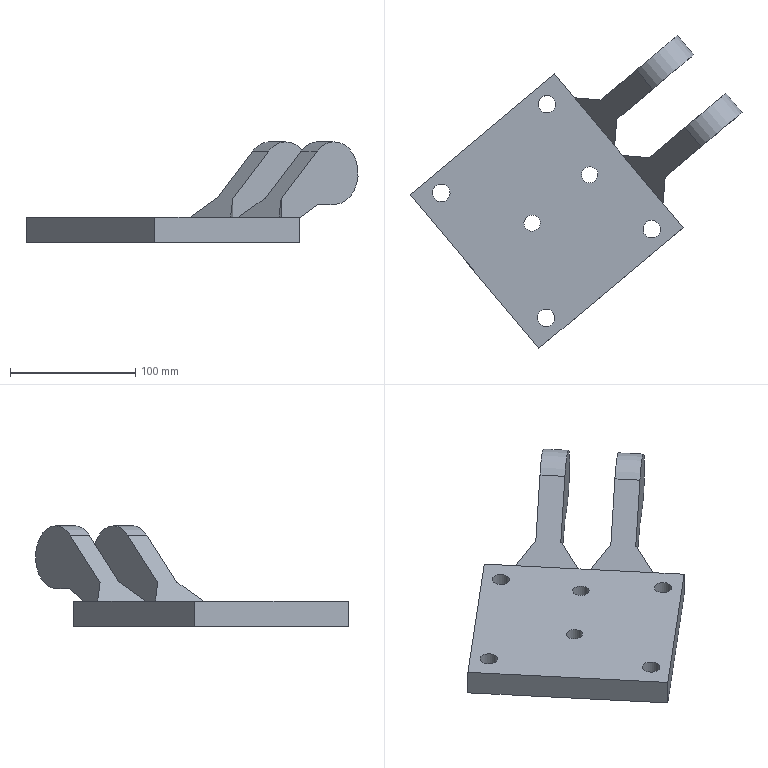Part | NX | features solid 2 | 1 solid | 30 faces | box 264.815 x 249.408 x 80 mm | volume 611339 mm3 | plane 22 | cylinder 8 | commonest cylinder face diameters 14 x4 13 x2 50 x2
STEP:
#1=CARTESIAN_POINT('',(922.471,361.992,-250.));
#2=VERTEX_POINT('',#1);
#3=CARTESIAN_POINT('',(906.401,381.143,-250.));
#4=VERTEX_POINT('',#3);
#5=CARTESIAN_POINT('',(977.108,296.878,-250.));
#6=DIRECTION('',(-0.6428,0.766,0.));
#7=VECTOR('',#6,1000.);
#8=LINE('',#5,#7);
#9=EDGE_CURVE('',#2,#4,#8,.T.);
#10=ORIENTED_EDGE('',*,*,#9,.T.);
#11=CARTESIAN_POINT('',(906.401,381.143,-230.));
#12=VERTEX_POINT('',#11);
#13=CARTESIAN_POINT('',(906.401,381.143,-230.));
#14=DIRECTION('',(0.,0.,1.));
#15=VECTOR('',#14,1000.);
#16=LINE('',#13,#15);
#17=EDGE_CURVE('',#4,#12,#16,.T.);
#18=ORIENTED_EDGE('',*,*,#17,.T.);
#19=CARTESIAN_POINT('',(922.471,361.992,-230.));
#20=VERTEX_POINT('',#19);
#21=CARTESIAN_POINT('',(977.108,296.878,-230.));
#22=DIRECTION('',(-0.6428,0.766,0.));
#23=VECTOR('',#22,1000.);
#24=LINE('',#21,#23);
#25=EDGE_CURVE('',#20,#12,#24,.T.);
#26=ORIENTED_EDGE('',*,*,#25,.F.);
#27=CARTESIAN_POINT('',(922.471,361.992,-230.));
#28=DIRECTION('',(0.,0.,-1.));
#29=VECTOR('',#28,1000.);
#30=LINE('',#27,#29);
#31=EDGE_CURVE('',#20,#2,#30,.T.);
#32=ORIENTED_EDGE('',*,*,#31,.T.);
#33=EDGE_LOOP('',(#10,#18,#26,#32));
#34=FACE_BOUND('',#33,.T.);
#35=CARTESIAN_POINT('',(977.108,296.878,-230.));
#36=DIRECTION('',(-0.766,-0.6428,0.));
#37=DIRECTION('',(0.,0.,-1.));
#38=AXIS2_PLACEMENT_3D('',#35,#36,#37);
#39=PLANE('',#38);
#40=ADVANCED_FACE('',(#34),#39,.F.);
#41=CARTESIAN_POINT('',(835.695,465.408,-230.));
#42=VERTEX_POINT('',#41);
#43=CARTESIAN_POINT('',(819.625,484.559,-230.));
#44=VERTEX_POINT('',#43);
#45=CARTESIAN_POINT('',(977.108,296.878,-230.));
#46=DIRECTION('',(-0.6428,0.766,0.));
#47=VECTOR('',#46,1000.);
#48=LINE('',#45,#47);
#49=EDGE_CURVE('',#42,#44,#48,.T.);
#50=ORIENTED_EDGE('',*,*,#49,.F.);
#51=CARTESIAN_POINT('',(835.695,465.408,-250.));
#52=VERTEX_POINT('',#51);
#53=CARTESIAN_POINT('',(835.695,465.408,-230.));
#54=DIRECTION('',(0.,0.,-1.));
#55=VECTOR('',#54,1000.);
#56=LINE('',#53,#55);
#57=EDGE_CURVE('',#42,#52,#56,.T.);
#58=ORIENTED_EDGE('',*,*,#57,.T.);
#59=CARTESIAN_POINT('',(819.625,484.559,-250.));
#60=VERTEX_POINT('',#59);
#61=CARTESIAN_POINT('',(977.108,296.878,-250.));
#62=DIRECTION('',(-0.6428,0.766,0.));
#63=VECTOR('',#62,1000.);
#64=LINE('',#61,#63);
#65=EDGE_CURVE('',#52,#60,#64,.T.);
#66=ORIENTED_EDGE('',*,*,#65,.T.);
#67=CARTESIAN_POINT('',(819.625,484.559,-230.));
#68=DIRECTION('',(0.,0.,-1.));
#69=VECTOR('',#68,1000.);
#70=LINE('',#67,#69);
#71=EDGE_CURVE('',#44,#60,#70,.T.);
#72=ORIENTED_EDGE('',*,*,#71,.F.);
#73=EDGE_LOOP('',(#50,#58,#66,#72));
#74=FACE_BOUND('',#73,.T.);
#75=CARTESIAN_POINT('',(977.108,296.878,-230.));
#76=DIRECTION('',(-0.766,-0.6428,0.));
#77=DIRECTION('',(0.,0.,-1.));
#78=AXIS2_PLACEMENT_3D('',#75,#76,#77);
#79=PLANE('',#78);
#80=ADVANCED_FACE('',(#74),#79,.F.);
#81=CARTESIAN_POINT('',(808.584,455.713,-230.));
#82=VERTEX_POINT('',#81);
#83=CARTESIAN_POINT('',(813.946,460.212,-230.));
#84=DIRECTION('',(0.,0.,1.));
#85=DIRECTION('',(-0.766,-0.6428,0.));
#86=AXIS2_PLACEMENT_3D('',#83,#84,#85);
#87=CIRCLE('',#86,7.);
#88=EDGE_CURVE('',#82,#82,#87,.T.);
#89=ORIENTED_EDGE('',*,*,#88,.F.);
#90=EDGE_LOOP('',(#89));
#91=FACE_BOUND('',#90,.T.);
#92=CARTESIAN_POINT('',(724.319,385.006,-230.));
#93=VERTEX_POINT('',#92);
#94=CARTESIAN_POINT('',(729.681,389.506,-230.));
#95=DIRECTION('',(0.,0.,1.));
#96=DIRECTION('',(-0.766,-0.6428,0.));
#97=AXIS2_PLACEMENT_3D('',#94,#95,#96);
#98=CIRCLE('',#97,7.);
#99=EDGE_CURVE('',#93,#93,#98,.T.);
#100=ORIENTED_EDGE('',*,*,#99,.F.);
#101=EDGE_LOOP('',(#100));
#102=FACE_BOUND('',#101,.T.);
#103=CARTESIAN_POINT('',(807.881,285.421,-230.));
#104=VERTEX_POINT('',#103);
#105=CARTESIAN_POINT('',(813.243,289.92,-230.));
#106=DIRECTION('',(0.,0.,1.));
#107=DIRECTION('',(-0.766,-0.6428,0.));
#108=AXIS2_PLACEMENT_3D('',#105,#106,#107);
#109=CIRCLE('',#108,7.);
#110=EDGE_CURVE('',#104,#104,#109,.T.);
#111=ORIENTED_EDGE('',*,*,#110,.F.);
#112=EDGE_LOOP('',(#111));
#113=FACE_BOUND('',#112,.T.);
#114=CARTESIAN_POINT('',(807.564,265.574,-230.));
#115=VERTEX_POINT('',#114);
#116=CARTESIAN_POINT('',(1251.87,638.39,-230.));
#117=DIRECTION('',(-0.766,-0.6428,0.));
#118=VECTOR('',#117,1000.);
#119=LINE('',#116,#118);
#120=EDGE_CURVE('',#20,#115,#119,.T.);
#121=ORIENTED_EDGE('',*,*,#120,.F.);
#122=ORIENTED_EDGE('',*,*,#25,.T.);
#123=CARTESIAN_POINT('',(874.262,419.445,-230.));
#124=VERTEX_POINT('',#123);
#125=CARTESIAN_POINT('',(896.759,392.634,-230.));
#126=DIRECTION('',(-0.6428,0.766,0.));
#127=VECTOR('',#126,1000.);
#128=LINE('',#125,#127);
#129=EDGE_CURVE('',#12,#124,#128,.T.);
#130=ORIENTED_EDGE('',*,*,#129,.T.);
#131=CARTESIAN_POINT('',(867.834,427.106,-230.));
#132=VERTEX_POINT('',#131);
#133=CARTESIAN_POINT('',(977.108,296.878,-230.));
#134=DIRECTION('',(-0.6428,0.766,0.));
#135=VECTOR('',#134,1000.);
#136=LINE('',#133,#135);
#137=EDGE_CURVE('',#124,#132,#136,.T.);
#138=ORIENTED_EDGE('',*,*,#137,.T.);
#139=CARTESIAN_POINT('',(858.192,438.596,-230.));
#140=DIRECTION('',(-0.6428,0.766,0.));
#141=VECTOR('',#140,1000.);
#142=LINE('',#139,#141);
#143=EDGE_CURVE('',#132,#42,#142,.T.);
#144=ORIENTED_EDGE('',*,*,#143,.T.);
#145=ORIENTED_EDGE('',*,*,#49,.T.);
#146=CARTESIAN_POINT('',(704.718,388.141,-230.));
#147=VERTEX_POINT('',#146);
#148=CARTESIAN_POINT('',(1149.024,760.958,-230.));
#149=DIRECTION('',(-0.766,-0.6428,0.));
#150=VECTOR('',#149,1000.);
#151=LINE('',#148,#150);
#152=EDGE_CURVE('',#44,#147,#151,.T.);
#153=ORIENTED_EDGE('',*,*,#152,.T.);
#154=CARTESIAN_POINT('',(862.201,200.46,-230.));
#155=DIRECTION('',(-0.6428,0.766,0.));
#156=VECTOR('',#155,1000.);
#157=LINE('',#154,#156);
#158=EDGE_CURVE('',#115,#147,#157,.T.);
#159=ORIENTED_EDGE('',*,*,#158,.F.);
#160=EDGE_LOOP('',(#121,#122,#130,#138,#144,#145,#153,#159));
#161=FACE_BOUND('',#160,.T.);
#162=CARTESIAN_POINT('',(797.125,361.246,-230.));
#163=VERTEX_POINT('',#162);
#164=CARTESIAN_POINT('',(802.104,365.424,-230.));
#165=DIRECTION('',(0.,0.,1.));
#166=DIRECTION('',(-0.766,-0.6428,0.));
#167=AXIS2_PLACEMENT_3D('',#164,#165,#166);
#168=CIRCLE('',#167,6.5);
#169=EDGE_CURVE('',#163,#163,#168,.T.);
#170=ORIENTED_EDGE('',*,*,#169,.F.);
#171=EDGE_LOOP('',(#170));
#172=FACE_BOUND('',#171,.T.);
#173=CARTESIAN_POINT('',(843.087,399.814,-230.));
#174=VERTEX_POINT('',#173);
#175=CARTESIAN_POINT('',(848.067,403.992,-230.));
#176=DIRECTION('',(0.,0.,1.));
#177=DIRECTION('',(-0.766,-0.6428,0.));
#178=AXIS2_PLACEMENT_3D('',#175,#176,#177);
#179=CIRCLE('',#178,6.5);
#180=EDGE_CURVE('',#174,#174,#179,.T.);
#181=ORIENTED_EDGE('',*,*,#180,.F.);
#182=EDGE_LOOP('',(#181));
#183=FACE_BOUND('',#182,.T.);
#184=CARTESIAN_POINT('',(892.146,356.127,-230.));
#185=VERTEX_POINT('',#184);
#186=CARTESIAN_POINT('',(897.508,360.627,-230.));
#187=DIRECTION('',(0.,0.,1.));
#188=DIRECTION('',(-0.766,-0.6428,0.));
#189=AXIS2_PLACEMENT_3D('',#186,#187,#188);
#190=CIRCLE('',#189,7.);
#191=EDGE_CURVE('',#185,#185,#190,.T.);
#192=ORIENTED_EDGE('',*,*,#191,.F.);
#193=EDGE_LOOP('',(#192));
#194=FACE_BOUND('',#193,.T.);
#195=CARTESIAN_POINT('',(1062.923,476.582,-230.));
#196=DIRECTION('',(0.,0.,1.));
#197=DIRECTION('',(-0.766,-0.6428,0.));
#198=AXIS2_PLACEMENT_3D('',#195,#196,#197);
#199=PLANE('',#198);
#200=ADVANCED_FACE('',(#91,#102,#113,#161,#172,#183,#194),#199,.T.);
#201=CARTESIAN_POINT('',(808.584,455.713,-250.));
#202=VERTEX_POINT('',#201);
#203=CARTESIAN_POINT('',(813.946,460.212,-250.));
#204=DIRECTION('',(0.,0.,1.));
#205=DIRECTION('',(-0.766,-0.6428,0.));
#206=AXIS2_PLACEMENT_3D('',#203,#204,#205);
#207=CIRCLE('',#206,7.);
#208=EDGE_CURVE('',#202,#202,#207,.T.);
#209=ORIENTED_EDGE('',*,*,#208,.T.);
#210=EDGE_LOOP('',(#209));
#211=FACE_BOUND('',#210,.T.);
#212=CARTESIAN_POINT('',(724.319,385.006,-250.));
#213=VERTEX_POINT('',#212);
#214=CARTESIAN_POINT('',(729.681,389.506,-250.));
#215=DIRECTION('',(0.,0.,1.));
#216=DIRECTION('',(-0.766,-0.6428,0.));
#217=AXIS2_PLACEMENT_3D('',#214,#215,#216);
#218=CIRCLE('',#217,7.);
#219=EDGE_CURVE('',#213,#213,#218,.T.);
#220=ORIENTED_EDGE('',*,*,#219,.T.);
#221=EDGE_LOOP('',(#220));
#222=FACE_BOUND('',#221,.T.);
#223=CARTESIAN_POINT('',(807.881,285.421,-250.));
#224=VERTEX_POINT('',#223);
#225=CARTESIAN_POINT('',(813.243,289.92,-250.));
#226=DIRECTION('',(0.,0.,1.));
#227=DIRECTION('',(-0.766,-0.6428,0.));
#228=AXIS2_PLACEMENT_3D('',#225,#226,#227);
#229=CIRCLE('',#228,7.);
#230=EDGE_CURVE('',#224,#224,#229,.T.);
#231=ORIENTED_EDGE('',*,*,#230,.T.);
#232=EDGE_LOOP('',(#231));
#233=FACE_BOUND('',#232,.T.);
#234=CARTESIAN_POINT('',(807.564,265.574,-250.));
#235=VERTEX_POINT('',#234);
#236=CARTESIAN_POINT('',(1251.87,638.39,-250.));
#237=DIRECTION('',(-0.766,-0.6428,0.));
#238=VECTOR('',#237,1000.);
#239=LINE('',#236,#238);
#240=EDGE_CURVE('',#2,#235,#239,.T.);
#241=ORIENTED_EDGE('',*,*,#240,.T.);
#242=CARTESIAN_POINT('',(704.718,388.141,-250.));
#243=VERTEX_POINT('',#242);
#244=CARTESIAN_POINT('',(862.201,200.46,-250.));
#245=DIRECTION('',(-0.6428,0.766,0.));
#246=VECTOR('',#245,1000.);
#247=LINE('',#244,#246);
#248=EDGE_CURVE('',#235,#243,#247,.T.);
#249=ORIENTED_EDGE('',*,*,#248,.T.);
#250=CARTESIAN_POINT('',(1149.024,760.958,-250.));
#251=DIRECTION('',(-0.766,-0.6428,0.));
#252=VECTOR('',#251,1000.);
#253=LINE('',#250,#252);
#254=EDGE_CURVE('',#60,#243,#253,.T.);
#255=ORIENTED_EDGE('',*,*,#254,.F.);
#256=ORIENTED_EDGE('',*,*,#65,.F.);
#257=CARTESIAN_POINT('',(867.834,427.106,-250.));
#258=VERTEX_POINT('',#257);
#259=CARTESIAN_POINT('',(858.192,438.596,-250.));
#260=DIRECTION('',(-0.6428,0.766,0.));
#261=VECTOR('',#260,1000.);
#262=LINE('',#259,#261);
#263=EDGE_CURVE('',#258,#52,#262,.T.);
#264=ORIENTED_EDGE('',*,*,#263,.F.);
#265=CARTESIAN_POINT('',(874.262,419.445,-250.));
#266=VERTEX_POINT('',#265);
#267=CARTESIAN_POINT('',(977.108,296.878,-250.));
#268=DIRECTION('',(-0.6428,0.766,0.));
#269=VECTOR('',#268,1000.);
#270=LINE('',#267,#269);
#271=EDGE_CURVE('',#266,#258,#270,.T.);
#272=ORIENTED_EDGE('',*,*,#271,.F.);
#273=CARTESIAN_POINT('',(896.759,392.634,-250.));
#274=DIRECTION('',(-0.6428,0.766,0.));
#275=VECTOR('',#274,1000.);
#276=LINE('',#273,#275);
#277=EDGE_CURVE('',#4,#266,#276,.T.);
#278=ORIENTED_EDGE('',*,*,#277,.F.);
#279=ORIENTED_EDGE('',*,*,#9,.F.);
#280=EDGE_LOOP('',(#241,#249,#255,#256,#264,#272,#278,#279));
#281=FACE_BOUND('',#280,.T.);
#282=CARTESIAN_POINT('',(797.125,361.246,-250.));
#283=VERTEX_POINT('',#282);
#284=CARTESIAN_POINT('',(802.104,365.424,-250.));
#285=DIRECTION('',(0.,0.,1.));
#286=DIRECTION('',(-0.766,-0.6428,0.));
#287=AXIS2_PLACEMENT_3D('',#284,#285,#286);
#288=CIRCLE('',#287,6.5);
#289=EDGE_CURVE('',#283,#283,#288,.T.);
#290=ORIENTED_EDGE('',*,*,#289,.T.);
#291=EDGE_LOOP('',(#290));
#292=FACE_BOUND('',#291,.T.);
#293=CARTESIAN_POINT('',(843.087,399.814,-250.));
#294=VERTEX_POINT('',#293);
#295=CARTESIAN_POINT('',(848.067,403.992,-250.));
#296=DIRECTION('',(0.,0.,1.));
#297=DIRECTION('',(-0.766,-0.6428,0.));
#298=AXIS2_PLACEMENT_3D('',#295,#296,#297);
#299=CIRCLE('',#298,6.5);
#300=EDGE_CURVE('',#294,#294,#299,.T.);
#301=ORIENTED_EDGE('',*,*,#300,.T.);
#302=EDGE_LOOP('',(#301));
#303=FACE_BOUND('',#302,.T.);
#304=CARTESIAN_POINT('',(892.146,356.127,-250.));
#305=VERTEX_POINT('',#304);
#306=CARTESIAN_POINT('',(897.508,360.627,-250.));
#307=DIRECTION('',(0.,0.,1.));
#308=DIRECTION('',(-0.766,-0.6428,0.));
#309=AXIS2_PLACEMENT_3D('',#306,#307,#308);
#310=CIRCLE('',#309,7.);
#311=EDGE_CURVE('',#305,#305,#310,.T.);
#312=ORIENTED_EDGE('',*,*,#311,.T.);
#313=EDGE_LOOP('',(#312));
#314=FACE_BOUND('',#313,.T.);
#315=CARTESIAN_POINT('',(1062.923,476.582,-250.));
#316=DIRECTION('',(0.,0.,1.));
#317=DIRECTION('',(-0.766,-0.6428,0.));
#318=AXIS2_PLACEMENT_3D('',#315,#316,#317);
#319=PLANE('',#318);
#320=ADVANCED_FACE('',(#211,#222,#233,#281,#292,#303,#314),#319,.F.);
#321=ORIENTED_EDGE('',*,*,#240,.F.);
#322=ORIENTED_EDGE('',*,*,#31,.F.);
#323=ORIENTED_EDGE('',*,*,#120,.T.);
#324=CARTESIAN_POINT('',(807.564,265.574,-230.));
#325=DIRECTION('',(0.,0.,-1.));
#326=VECTOR('',#325,1000.);
#327=LINE('',#324,#326);
#328=EDGE_CURVE('',#115,#235,#327,.T.);
#329=ORIENTED_EDGE('',*,*,#328,.T.);
#330=EDGE_LOOP('',(#321,#322,#323,#329));
#331=FACE_BOUND('',#330,.T.);
#332=CARTESIAN_POINT('',(1251.87,638.39,-230.));
#333=DIRECTION('',(0.6428,-0.766,0.));
#334=DIRECTION('',(0.,0.,1.));
#335=AXIS2_PLACEMENT_3D('',#332,#333,#334);
#336=PLANE('',#335);
#337=ADVANCED_FACE('',(#331),#336,.T.);
#338=ORIENTED_EDGE('',*,*,#137,.F.);
#339=CARTESIAN_POINT('',(874.262,419.445,-230.));
#340=DIRECTION('',(0.,0.,-1.));
#341=VECTOR('',#340,1000.);
#342=LINE('',#339,#341);
#343=EDGE_CURVE('',#124,#266,#342,.T.);
#344=ORIENTED_EDGE('',*,*,#343,.T.);
#345=ORIENTED_EDGE('',*,*,#271,.T.);
#346=CARTESIAN_POINT('',(867.834,427.106,-230.));
#347=DIRECTION('',(0.,0.,1.));
#348=VECTOR('',#347,1000.);
#349=LINE('',#346,#348);
#350=EDGE_CURVE('',#258,#132,#349,.T.);
#351=ORIENTED_EDGE('',*,*,#350,.T.);
#352=EDGE_LOOP('',(#338,#344,#345,#351));
#353=FACE_BOUND('',#352,.T.);
#354=CARTESIAN_POINT('',(977.108,296.878,-230.));
#355=DIRECTION('',(-0.766,-0.6428,0.));
#356=DIRECTION('',(0.,0.,-1.));
#357=AXIS2_PLACEMENT_3D('',#354,#355,#356);
#358=PLANE('',#357);
#359=ADVANCED_FACE('',(#353),#358,.F.);
#360=ORIENTED_EDGE('',*,*,#254,.T.);
#361=CARTESIAN_POINT('',(704.718,388.141,-230.));
#362=DIRECTION('',(0.,0.,-1.));
#363=VECTOR('',#362,1000.);
#364=LINE('',#361,#363);
#365=EDGE_CURVE('',#147,#243,#364,.T.);
#366=ORIENTED_EDGE('',*,*,#365,.F.);
#367=ORIENTED_EDGE('',*,*,#152,.F.);
#368=ORIENTED_EDGE('',*,*,#71,.T.);
#369=EDGE_LOOP('',(#360,#366,#367,#368));
#370=FACE_BOUND('',#369,.T.);
#371=CARTESIAN_POINT('',(1149.024,760.958,-230.));
#372=DIRECTION('',(0.6428,-0.766,0.));
#373=DIRECTION('',(0.,0.,1.));
#374=AXIS2_PLACEMENT_3D('',#371,#372,#373);
#375=PLANE('',#374);
#376=ADVANCED_FACE('',(#370),#375,.F.);
#377=ORIENTED_EDGE('',*,*,#248,.F.);
#378=ORIENTED_EDGE('',*,*,#328,.F.);
#379=ORIENTED_EDGE('',*,*,#158,.T.);
#380=ORIENTED_EDGE('',*,*,#365,.T.);
#381=EDGE_LOOP('',(#377,#378,#379,#380));
#382=FACE_BOUND('',#381,.T.);
#383=CARTESIAN_POINT('',(862.201,200.46,-230.));
#384=DIRECTION('',(-0.766,-0.6428,0.));
#385=DIRECTION('',(0.,0.,-1.));
#386=AXIS2_PLACEMENT_3D('',#383,#384,#385);
#387=PLANE('',#386);
#388=ADVANCED_FACE('',(#382),#387,.T.);
#389=ORIENTED_EDGE('',*,*,#110,.T.);
#390=EDGE_LOOP('',(#389));
#391=FACE_BOUND('',#390,.T.);
#392=ORIENTED_EDGE('',*,*,#230,.F.);
#393=EDGE_LOOP('',(#392));
#394=FACE_BOUND('',#393,.T.);
#395=CARTESIAN_POINT('',(813.243,289.92,-230.));
#396=DIRECTION('',(0.,0.,-1.));
#397=DIRECTION('',(0.766,0.6428,0.));
#398=AXIS2_PLACEMENT_3D('',#395,#396,#397);
#399=CYLINDRICAL_SURFACE('',#398,7.);
#400=ADVANCED_FACE('',(#391,#394),#399,.F.);
#401=ORIENTED_EDGE('',*,*,#169,.T.);
#402=EDGE_LOOP('',(#401));
#403=FACE_BOUND('',#402,.T.);
#404=ORIENTED_EDGE('',*,*,#289,.F.);
#405=EDGE_LOOP('',(#404));
#406=FACE_BOUND('',#405,.T.);
#407=CARTESIAN_POINT('',(802.104,365.424,-230.));
#408=DIRECTION('',(0.,0.,-1.));
#409=DIRECTION('',(0.766,0.6428,0.));
#410=AXIS2_PLACEMENT_3D('',#407,#408,#409);
#411=CYLINDRICAL_SURFACE('',#410,6.5);
#412=ADVANCED_FACE('',(#403,#406),#411,.F.);
#413=ORIENTED_EDGE('',*,*,#99,.T.);
#414=EDGE_LOOP('',(#413));
#415=FACE_BOUND('',#414,.T.);
#416=ORIENTED_EDGE('',*,*,#219,.F.);
#417=EDGE_LOOP('',(#416));
#418=FACE_BOUND('',#417,.T.);
#419=CARTESIAN_POINT('',(729.681,389.506,-230.));
#420=DIRECTION('',(0.,0.,-1.));
#421=DIRECTION('',(0.766,0.6428,0.));
#422=AXIS2_PLACEMENT_3D('',#419,#420,#421);
#423=CYLINDRICAL_SURFACE('',#422,7.);
#424=ADVANCED_FACE('',(#415,#418),#423,.F.);
#425=ORIENTED_EDGE('',*,*,#180,.T.);
#426=EDGE_LOOP('',(#425));
#427=FACE_BOUND('',#426,.T.);
#428=ORIENTED_EDGE('',*,*,#300,.F.);
#429=EDGE_LOOP('',(#428));
#430=FACE_BOUND('',#429,.T.);
#431=CARTESIAN_POINT('',(848.067,403.992,-230.));
#432=DIRECTION('',(0.,0.,-1.));
#433=DIRECTION('',(0.766,0.6428,0.));
#434=AXIS2_PLACEMENT_3D('',#431,#432,#433);
#435=CYLINDRICAL_SURFACE('',#434,6.5);
#436=ADVANCED_FACE('',(#427,#430),#435,.F.);
#437=ORIENTED_EDGE('',*,*,#88,.T.);
#438=EDGE_LOOP('',(#437));
#439=FACE_BOUND('',#438,.T.);
#440=ORIENTED_EDGE('',*,*,#208,.F.);
#441=EDGE_LOOP('',(#440));
#442=FACE_BOUND('',#441,.T.);
#443=CARTESIAN_POINT('',(813.946,460.212,-230.));
#444=DIRECTION('',(0.,0.,-1.));
#445=DIRECTION('',(0.766,0.6428,0.));
#446=AXIS2_PLACEMENT_3D('',#443,#444,#445);
#447=CYLINDRICAL_SURFACE('',#446,7.);
#448=ADVANCED_FACE('',(#439,#442),#447,.F.);
#449=ORIENTED_EDGE('',*,*,#191,.T.);
#450=EDGE_LOOP('',(#449));
#451=FACE_BOUND('',#450,.T.);
#452=ORIENTED_EDGE('',*,*,#311,.F.);
#453=EDGE_LOOP('',(#452));
#454=FACE_BOUND('',#453,.T.);
#455=CARTESIAN_POINT('',(897.508,360.627,-230.));
#456=DIRECTION('',(0.,0.,-1.));
#457=DIRECTION('',(0.766,0.6428,0.));
#458=AXIS2_PLACEMENT_3D('',#455,#456,#457);
#459=CYLINDRICAL_SURFACE('',#458,7.);
#460=ADVANCED_FACE('',(#451,#454),#459,.F.);
#461=CARTESIAN_POINT('',(911.815,483.591,-220.));
#462=VERTEX_POINT('',#461);
#463=CARTESIAN_POINT('',(898.96,498.912,-220.));
#464=VERTEX_POINT('',#463);
#465=CARTESIAN_POINT('',(911.815,483.591,-220.));
#466=DIRECTION('',(-0.6428,0.766,0.));
#467=VECTOR('',#466,1000.);
#468=LINE('',#465,#467);
#469=EDGE_CURVE('',#462,#464,#468,.T.);
#470=ORIENTED_EDGE('',*,*,#469,.T.);
#471=CARTESIAN_POINT('',(885.372,487.511,-177.382));
#472=VERTEX_POINT('',#471);
#473=CARTESIAN_POINT('',(898.96,498.912,-195.));
#474=DIRECTION('',(-0.6428,0.766,0.));
#475=DIRECTION('',(-0.766,-0.6428,0.));
#476=AXIS2_PLACEMENT_3D('',#473,#474,#475);
#477=CIRCLE('',#476,25.);
#478=EDGE_CURVE('',#472,#464,#477,.T.);
#479=ORIENTED_EDGE('',*,*,#478,.F.);
#480=CARTESIAN_POINT('',(898.228,472.19,-177.382));
#481=VERTEX_POINT('',#480);
#482=CARTESIAN_POINT('',(898.228,472.19,-177.382));
#483=DIRECTION('',(-0.6428,0.766,0.));
#484=VECTOR('',#483,1000.);
#485=LINE('',#482,#484);
#486=EDGE_CURVE('',#481,#472,#485,.T.);
#487=ORIENTED_EDGE('',*,*,#486,.F.);
#488=CARTESIAN_POINT('',(911.815,483.591,-195.));
#489=DIRECTION('',(-0.6428,0.766,0.));
#490=DIRECTION('',(-0.766,-0.6428,0.));
#491=AXIS2_PLACEMENT_3D('',#488,#489,#490);
#492=CIRCLE('',#491,25.);
#493=EDGE_CURVE('',#481,#462,#492,.T.);
#494=ORIENTED_EDGE('',*,*,#493,.T.);
#495=EDGE_LOOP('',(#470,#479,#487,#494));
#496=FACE_BOUND('',#495,.T.);
#497=CARTESIAN_POINT('',(911.815,483.591,-195.));
#498=DIRECTION('',(-0.6428,0.766,0.));
#499=DIRECTION('',(0.,0.,-1.));
#500=AXIS2_PLACEMENT_3D('',#497,#498,#499);
#501=CYLINDRICAL_SURFACE('',#500,25.);
#502=ADVANCED_FACE('',(#496),#501,.T.);
#503=CARTESIAN_POINT('',(869.683,448.238,-214.898));
#504=VERTEX_POINT('',#503);
#505=CARTESIAN_POINT('',(858.192,438.596,-230.));
#506=DIRECTION('',(0.5398,0.453,0.7095));
#507=VECTOR('',#506,1000.);
#508=LINE('',#505,#507);
#509=EDGE_CURVE('',#504,#481,#508,.T.);
#510=ORIENTED_EDGE('',*,*,#509,.F.);
#511=CARTESIAN_POINT('',(869.683,448.238,-241.499));
#512=VERTEX_POINT('',#511);
#513=CARTESIAN_POINT('',(869.683,448.238,-250.));
#514=DIRECTION('',(0.,0.,-1.));
#515=VECTOR('',#514,1000.);
#516=LINE('',#513,#515);
#517=EDGE_CURVE('',#504,#512,#516,.T.);
#518=ORIENTED_EDGE('',*,*,#517,.T.);
#519=CARTESIAN_POINT('',(898.744,472.623,-220.));
#520=VERTEX_POINT('',#519);
#521=CARTESIAN_POINT('',(898.744,472.623,-220.));
#522=DIRECTION('',(-0.6665,-0.5592,-0.493));
#523=VECTOR('',#522,1000.);
#524=LINE('',#521,#523);
#525=EDGE_CURVE('',#520,#512,#524,.T.);
#526=ORIENTED_EDGE('',*,*,#525,.F.);
#527=CARTESIAN_POINT('',(911.815,483.591,-220.));
#528=DIRECTION('',(-0.766,-0.6428,0.));
#529=VECTOR('',#528,1000.);
#530=LINE('',#527,#529);
#531=EDGE_CURVE('',#462,#520,#530,.T.);
#532=ORIENTED_EDGE('',*,*,#531,.F.);
#533=ORIENTED_EDGE('',*,*,#493,.F.);
#534=EDGE_LOOP('',(#510,#518,#526,#532,#533));
#535=FACE_BOUND('',#534,.T.);
#536=CARTESIAN_POINT('',(911.815,483.591,-195.));
#537=DIRECTION('',(-0.6428,0.766,0.));
#538=DIRECTION('',(0.,0.,-1.));
#539=AXIS2_PLACEMENT_3D('',#536,#537,#538);
#540=PLANE('',#539);
#541=ADVANCED_FACE('',(#535),#540,.F.);
#542=CARTESIAN_POINT('',(885.888,487.944,-220.));
#543=VERTEX_POINT('',#542);
#544=CARTESIAN_POINT('',(856.827,463.559,-241.499));
#545=VERTEX_POINT('',#544);
#546=CARTESIAN_POINT('',(885.888,487.944,-220.));
#547=DIRECTION('',(-0.6665,-0.5592,-0.493));
#548=VECTOR('',#547,1000.);
#549=LINE('',#546,#548);
#550=EDGE_CURVE('',#543,#545,#549,.T.);
#551=ORIENTED_EDGE('',*,*,#550,.T.);
#552=CARTESIAN_POINT('',(856.827,463.559,-214.898));
#553=VERTEX_POINT('',#552);
#554=CARTESIAN_POINT('',(856.827,463.559,-195.));
#555=DIRECTION('',(0.,0.,1.));
#556=VECTOR('',#555,1000.);
#557=LINE('',#554,#556);
#558=EDGE_CURVE('',#545,#553,#557,.T.);
#559=ORIENTED_EDGE('',*,*,#558,.T.);
#560=CARTESIAN_POINT('',(845.336,453.917,-230.));
#561=DIRECTION('',(0.5398,0.453,0.7095));
#562=VECTOR('',#561,1000.);
#563=LINE('',#560,#562);
#564=EDGE_CURVE('',#553,#472,#563,.T.);
#565=ORIENTED_EDGE('',*,*,#564,.T.);
#566=ORIENTED_EDGE('',*,*,#478,.T.);
#567=CARTESIAN_POINT('',(898.96,498.912,-220.));
#568=DIRECTION('',(-0.766,-0.6428,0.));
#569=VECTOR('',#568,1000.);
#570=LINE('',#567,#569);
#571=EDGE_CURVE('',#464,#543,#570,.T.);
#572=ORIENTED_EDGE('',*,*,#571,.T.);
#573=EDGE_LOOP('',(#551,#559,#565,#566,#572));
#574=FACE_BOUND('',#573,.T.);
#575=CARTESIAN_POINT('',(898.96,498.912,-195.));
#576=DIRECTION('',(-0.6428,0.766,0.));
#577=DIRECTION('',(0.,0.,-1.));
#578=AXIS2_PLACEMENT_3D('',#575,#576,#577);
#579=PLANE('',#578);
#580=ADVANCED_FACE('',(#574),#579,.T.);
#581=ORIENTED_EDGE('',*,*,#571,.F.);
#582=ORIENTED_EDGE('',*,*,#469,.F.);
#583=ORIENTED_EDGE('',*,*,#531,.T.);
#584=CARTESIAN_POINT('',(898.744,472.623,-220.));
#585=DIRECTION('',(-0.6428,0.766,0.));
#586=VECTOR('',#585,1000.);
#587=LINE('',#584,#586);
#588=EDGE_CURVE('',#520,#543,#587,.T.);
#589=ORIENTED_EDGE('',*,*,#588,.T.);
#590=EDGE_LOOP('',(#581,#582,#583,#589));
#591=FACE_BOUND('',#590,.T.);
#592=CARTESIAN_POINT('',(911.815,483.591,-220.));
#593=DIRECTION('',(0.,0.,-1.));
#594=DIRECTION('',(0.766,0.6428,0.));
#595=AXIS2_PLACEMENT_3D('',#592,#593,#594);
#596=PLANE('',#595);
#597=ADVANCED_FACE('',(#591),#596,.T.);
#598=ORIENTED_EDGE('',*,*,#550,.F.);
#599=ORIENTED_EDGE('',*,*,#588,.F.);
#600=ORIENTED_EDGE('',*,*,#525,.T.);
#601=CARTESIAN_POINT('',(868.436,433.985,-247.233));
#602=DIRECTION('',(0.0809,0.9247,0.372));
#603=VECTOR('',#602,1000.);
#604=LINE('',#601,#603);
#605=EDGE_CURVE('',#512,#258,#604,.F.);
#606=ORIENTED_EDGE('',*,*,#605,.T.);
#607=ORIENTED_EDGE('',*,*,#263,.T.);
#608=CARTESIAN_POINT('',(872.821,462.16,-235.066));
#609=DIRECTION('',(0.9247,-0.0809,0.372));
#610=VECTOR('',#609,1000.);
#611=LINE('',#608,#610);
#612=EDGE_CURVE('',#52,#545,#611,.T.);
#613=ORIENTED_EDGE('',*,*,#612,.T.);
#614=EDGE_LOOP('',(#598,#599,#600,#606,#607,#613));
#615=FACE_BOUND('',#614,.T.);
#616=CARTESIAN_POINT('',(898.744,472.623,-220.));
#617=DIRECTION('',(0.3777,0.3169,-0.87));
#618=DIRECTION('',(0.6665,0.5592,0.493));
#619=AXIS2_PLACEMENT_3D('',#616,#617,#618);
#620=PLANE('',#619);
#621=ADVANCED_FACE('',(#615),#620,.T.);
#622=ORIENTED_EDGE('',*,*,#564,.F.);
#623=CARTESIAN_POINT('',(866.192,462.74,-208.205));
#624=DIRECTION('',(-0.8115,0.071,-0.58));
#625=VECTOR('',#624,1000.);
#626=LINE('',#623,#625);
#627=EDGE_CURVE('',#553,#42,#626,.T.);
#628=ORIENTED_EDGE('',*,*,#627,.T.);
#629=ORIENTED_EDGE('',*,*,#143,.F.);
#630=CARTESIAN_POINT('',(867.834,427.106,-230.));
#631=DIRECTION('',(-0.071,-0.8115,-0.58));
#632=VECTOR('',#631,1000.);
#633=LINE('',#630,#632);
#634=EDGE_CURVE('',#132,#504,#633,.F.);
#635=ORIENTED_EDGE('',*,*,#634,.T.);
#636=ORIENTED_EDGE('',*,*,#509,.T.);
#637=ORIENTED_EDGE('',*,*,#486,.T.);
#638=EDGE_LOOP('',(#622,#628,#629,#635,#636,#637));
#639=FACE_BOUND('',#638,.T.);
#640=CARTESIAN_POINT('',(858.192,438.596,-230.));
#641=DIRECTION('',(-0.5435,-0.4561,0.7047));
#642=DIRECTION('',(-0.5398,-0.453,-0.7095));
#643=AXIS2_PLACEMENT_3D('',#640,#641,#642);
#644=PLANE('',#643);
#645=ADVANCED_FACE('',(#639),#644,.T.);
#646=CARTESIAN_POINT('',(950.383,437.629,-220.));
#647=VERTEX_POINT('',#646);
#648=CARTESIAN_POINT('',(937.527,452.95,-220.));
#649=VERTEX_POINT('',#648);
#650=CARTESIAN_POINT('',(950.383,437.629,-220.));
#651=DIRECTION('',(-0.6428,0.766,0.));
#652=VECTOR('',#651,1000.);
#653=LINE('',#650,#652);
#654=EDGE_CURVE('',#647,#649,#653,.T.);
#655=ORIENTED_EDGE('',*,*,#654,.T.);
#656=CARTESIAN_POINT('',(923.939,441.548,-177.382));
#657=VERTEX_POINT('',#656);
#658=CARTESIAN_POINT('',(937.527,452.95,-195.));
#659=DIRECTION('',(-0.6428,0.766,0.));
#660=DIRECTION('',(-0.766,-0.6428,0.));
#661=AXIS2_PLACEMENT_3D('',#658,#659,#660);
#662=CIRCLE('',#661,25.);
#663=EDGE_CURVE('',#657,#649,#662,.T.);
#664=ORIENTED_EDGE('',*,*,#663,.F.);
#665=CARTESIAN_POINT('',(936.795,426.227,-177.382));
#666=VERTEX_POINT('',#665);
#667=CARTESIAN_POINT('',(936.795,426.227,-177.382));
#668=DIRECTION('',(-0.6428,0.766,0.));
#669=VECTOR('',#668,1000.);
#670=LINE('',#667,#669);
#671=EDGE_CURVE('',#666,#657,#670,.T.);
#672=ORIENTED_EDGE('',*,*,#671,.F.);
#673=CARTESIAN_POINT('',(950.383,437.629,-195.));
#674=DIRECTION('',(-0.6428,0.766,0.));
#675=DIRECTION('',(-0.766,-0.6428,0.));
#676=AXIS2_PLACEMENT_3D('',#673,#674,#675);
#677=CIRCLE('',#676,25.);
#678=EDGE_CURVE('',#666,#647,#677,.T.);
#679=ORIENTED_EDGE('',*,*,#678,.T.);
#680=EDGE_LOOP('',(#655,#664,#672,#679));
#681=FACE_BOUND('',#680,.T.);
#682=CARTESIAN_POINT('',(950.383,437.629,-195.));
#683=DIRECTION('',(-0.6428,0.766,0.));
#684=DIRECTION('',(0.,0.,-1.));
#685=AXIS2_PLACEMENT_3D('',#682,#683,#684);
#686=CYLINDRICAL_SURFACE('',#685,25.);
#687=ADVANCED_FACE('',(#681),#686,.T.);
#688=CARTESIAN_POINT('',(908.25,402.275,-214.898));
#689=VERTEX_POINT('',#688);
#690=CARTESIAN_POINT('',(896.759,392.634,-230.));
#691=DIRECTION('',(0.5398,0.453,0.7095));
#692=VECTOR('',#691,1000.);
#693=LINE('',#690,#692);
#694=EDGE_CURVE('',#689,#666,#693,.T.);
#695=ORIENTED_EDGE('',*,*,#694,.F.);
#696=CARTESIAN_POINT('',(908.25,402.275,-241.499));
#697=VERTEX_POINT('',#696);
#698=CARTESIAN_POINT('',(908.25,402.275,-250.));
#699=DIRECTION('',(0.,0.,-1.));
#700=VECTOR('',#699,1000.);
#701=LINE('',#698,#700);
#702=EDGE_CURVE('',#689,#697,#701,.T.);
#703=ORIENTED_EDGE('',*,*,#702,.T.);
#704=CARTESIAN_POINT('',(937.311,426.661,-220.));
#705=VERTEX_POINT('',#704);
#706=CARTESIAN_POINT('',(937.311,426.661,-220.));
#707=DIRECTION('',(-0.6665,-0.5592,-0.493));
#708=VECTOR('',#707,1000.);
#709=LINE('',#706,#708);
#710=EDGE_CURVE('',#705,#697,#709,.T.);
#711=ORIENTED_EDGE('',*,*,#710,.F.);
#712=CARTESIAN_POINT('',(950.383,437.629,-220.));
#713=DIRECTION('',(-0.766,-0.6428,0.));
#714=VECTOR('',#713,1000.);
#715=LINE('',#712,#714);
#716=EDGE_CURVE('',#647,#705,#715,.T.);
#717=ORIENTED_EDGE('',*,*,#716,.F.);
#718=ORIENTED_EDGE('',*,*,#678,.F.);
#719=EDGE_LOOP('',(#695,#703,#711,#717,#718));
#720=FACE_BOUND('',#719,.T.);
#721=CARTESIAN_POINT('',(950.383,437.629,-195.));
#722=DIRECTION('',(-0.6428,0.766,0.));
#723=DIRECTION('',(0.,0.,-1.));
#724=AXIS2_PLACEMENT_3D('',#721,#722,#723);
#725=PLANE('',#724);
#726=ADVANCED_FACE('',(#720),#725,.F.);
#727=CARTESIAN_POINT('',(924.456,441.982,-220.));
#728=VERTEX_POINT('',#727);
#729=CARTESIAN_POINT('',(895.394,417.596,-241.499));
#730=VERTEX_POINT('',#729);
#731=CARTESIAN_POINT('',(924.456,441.982,-220.));
#732=DIRECTION('',(-0.6665,-0.5592,-0.493));
#733=VECTOR('',#732,1000.);
#734=LINE('',#731,#733);
#735=EDGE_CURVE('',#728,#730,#734,.T.);
#736=ORIENTED_EDGE('',*,*,#735,.T.);
#737=CARTESIAN_POINT('',(895.394,417.596,-214.898));
#738=VERTEX_POINT('',#737);
#739=CARTESIAN_POINT('',(895.394,417.596,-195.));
#740=DIRECTION('',(0.,0.,1.));
#741=VECTOR('',#740,1000.);
#742=LINE('',#739,#741);
#743=EDGE_CURVE('',#730,#738,#742,.T.);
#744=ORIENTED_EDGE('',*,*,#743,.T.);
#745=CARTESIAN_POINT('',(883.904,407.954,-230.));
#746=DIRECTION('',(0.5398,0.453,0.7095));
#747=VECTOR('',#746,1000.);
#748=LINE('',#745,#747);
#749=EDGE_CURVE('',#738,#657,#748,.T.);
#750=ORIENTED_EDGE('',*,*,#749,.T.);
#751=ORIENTED_EDGE('',*,*,#663,.T.);
#752=CARTESIAN_POINT('',(937.527,452.95,-220.));
#753=DIRECTION('',(-0.766,-0.6428,0.));
#754=VECTOR('',#753,1000.);
#755=LINE('',#752,#754);
#756=EDGE_CURVE('',#649,#728,#755,.T.);
#757=ORIENTED_EDGE('',*,*,#756,.T.);
#758=EDGE_LOOP('',(#736,#744,#750,#751,#757));
#759=FACE_BOUND('',#758,.T.);
#760=CARTESIAN_POINT('',(937.527,452.95,-195.));
#761=DIRECTION('',(-0.6428,0.766,0.));
#762=DIRECTION('',(0.,0.,-1.));
#763=AXIS2_PLACEMENT_3D('',#760,#761,#762);
#764=PLANE('',#763);
#765=ADVANCED_FACE('',(#759),#764,.T.);
#766=ORIENTED_EDGE('',*,*,#756,.F.);
#767=ORIENTED_EDGE('',*,*,#654,.F.);
#768=ORIENTED_EDGE('',*,*,#716,.T.);
#769=CARTESIAN_POINT('',(937.311,426.661,-220.));
#770=DIRECTION('',(-0.6428,0.766,0.));
#771=VECTOR('',#770,1000.);
#772=LINE('',#769,#771);
#773=EDGE_CURVE('',#705,#728,#772,.T.);
#774=ORIENTED_EDGE('',*,*,#773,.T.);
#775=EDGE_LOOP('',(#766,#767,#768,#774));
#776=FACE_BOUND('',#775,.T.);
#777=CARTESIAN_POINT('',(950.383,437.629,-220.));
#778=DIRECTION('',(0.,0.,-1.));
#779=DIRECTION('',(0.766,0.6428,0.));
#780=AXIS2_PLACEMENT_3D('',#777,#778,#779);
#781=PLANE('',#780);
#782=ADVANCED_FACE('',(#776),#781,.T.);
#783=ORIENTED_EDGE('',*,*,#735,.F.);
#784=ORIENTED_EDGE('',*,*,#773,.F.);
#785=ORIENTED_EDGE('',*,*,#710,.T.);
#786=CARTESIAN_POINT('',(907.003,388.022,-247.233));
#787=DIRECTION('',(0.0809,0.9247,0.372));
#788=VECTOR('',#787,1000.);
#789=LINE('',#786,#788);
#790=EDGE_CURVE('',#697,#4,#789,.F.);
#791=ORIENTED_EDGE('',*,*,#790,.T.);
#792=ORIENTED_EDGE('',*,*,#277,.T.);
#793=CARTESIAN_POINT('',(911.389,416.197,-235.066));
#794=DIRECTION('',(0.9247,-0.0809,0.372));
#795=VECTOR('',#794,1000.);
#796=LINE('',#793,#795);
#797=EDGE_CURVE('',#266,#730,#796,.T.);
#798=ORIENTED_EDGE('',*,*,#797,.T.);
#799=EDGE_LOOP('',(#783,#784,#785,#791,#792,#798));
#800=FACE_BOUND('',#799,.T.);
#801=CARTESIAN_POINT('',(937.311,426.661,-220.));
#802=DIRECTION('',(0.3777,0.3169,-0.87));
#803=DIRECTION('',(0.6665,0.5592,0.493));
#804=AXIS2_PLACEMENT_3D('',#801,#802,#803);
#805=PLANE('',#804);
#806=ADVANCED_FACE('',(#800),#805,.T.);
#807=ORIENTED_EDGE('',*,*,#749,.F.);
#808=CARTESIAN_POINT('',(904.76,416.777,-208.205));
#809=DIRECTION('',(-0.8115,0.071,-0.58));
#810=VECTOR('',#809,1000.);
#811=LINE('',#808,#810);
#812=EDGE_CURVE('',#738,#124,#811,.T.);
#813=ORIENTED_EDGE('',*,*,#812,.T.);
#814=ORIENTED_EDGE('',*,*,#129,.F.);
#815=CARTESIAN_POINT('',(906.401,381.143,-230.));
#816=DIRECTION('',(-0.071,-0.8115,-0.58));
#817=VECTOR('',#816,1000.);
#818=LINE('',#815,#817);
#819=EDGE_CURVE('',#12,#689,#818,.F.);
#820=ORIENTED_EDGE('',*,*,#819,.T.);
#821=ORIENTED_EDGE('',*,*,#694,.T.);
#822=ORIENTED_EDGE('',*,*,#671,.T.);
#823=EDGE_LOOP('',(#807,#813,#814,#820,#821,#822));
#824=FACE_BOUND('',#823,.T.);
#825=CARTESIAN_POINT('',(896.759,392.634,-230.));
#826=DIRECTION('',(-0.5435,-0.4561,0.7047));
#827=DIRECTION('',(-0.5398,-0.453,-0.7095));
#828=AXIS2_PLACEMENT_3D('',#825,#826,#827);
#829=PLANE('',#828);
#830=ADVANCED_FACE('',(#824),#829,.T.);
#831=ORIENTED_EDGE('',*,*,#612,.F.);
#832=ORIENTED_EDGE('',*,*,#57,.F.);
#833=ORIENTED_EDGE('',*,*,#627,.F.);
#834=ORIENTED_EDGE('',*,*,#558,.F.);
#835=EDGE_LOOP('',(#831,#832,#833,#834));
#836=FACE_BOUND('',#835,.T.);
#837=CARTESIAN_POINT('',(856.827,463.559,-195.));
#838=DIRECTION('',(-0.08716,-0.9962,0.));
#839=DIRECTION('',(0.9962,-0.08716,0.));
#840=AXIS2_PLACEMENT_3D('',#837,#838,#839);
#841=PLANE('',#840);
#842=ADVANCED_FACE('',(#836),#841,.F.);
#843=ORIENTED_EDGE('',*,*,#605,.F.);
#844=ORIENTED_EDGE('',*,*,#517,.F.);
#845=ORIENTED_EDGE('',*,*,#634,.F.);
#846=ORIENTED_EDGE('',*,*,#350,.F.);
#847=EDGE_LOOP('',(#843,#844,#845,#846));
#848=FACE_BOUND('',#847,.T.);
#849=CARTESIAN_POINT('',(867.834,427.106,-230.));
#850=DIRECTION('',(0.9962,-0.08716,0.));
#851=DIRECTION('',(0.08716,0.9962,0.));
#852=AXIS2_PLACEMENT_3D('',#849,#850,#851);
#853=PLANE('',#852);
#854=ADVANCED_FACE('',(#848),#853,.T.);
#855=ORIENTED_EDGE('',*,*,#797,.F.);
#856=ORIENTED_EDGE('',*,*,#343,.F.);
#857=ORIENTED_EDGE('',*,*,#812,.F.);
#858=ORIENTED_EDGE('',*,*,#743,.F.);
#859=EDGE_LOOP('',(#855,#856,#857,#858));
#860=FACE_BOUND('',#859,.T.);
#861=CARTESIAN_POINT('',(895.394,417.596,-195.));
#862=DIRECTION('',(-0.08716,-0.9962,0.));
#863=DIRECTION('',(0.9962,-0.08716,0.));
#864=AXIS2_PLACEMENT_3D('',#861,#862,#863);
#865=PLANE('',#864);
#866=ADVANCED_FACE('',(#860),#865,.F.);
#867=ORIENTED_EDGE('',*,*,#790,.F.);
#868=ORIENTED_EDGE('',*,*,#702,.F.);
#869=ORIENTED_EDGE('',*,*,#819,.F.);
#870=ORIENTED_EDGE('',*,*,#17,.F.);
#871=EDGE_LOOP('',(#867,#868,#869,#870));
#872=FACE_BOUND('',#871,.T.);
#873=CARTESIAN_POINT('',(906.401,381.143,-230.));
#874=DIRECTION('',(0.9962,-0.08716,0.));
#875=DIRECTION('',(0.08716,0.9962,0.));
#876=AXIS2_PLACEMENT_3D('',#873,#874,#875);
#877=PLANE('',#876);
#878=ADVANCED_FACE('',(#872),#877,.T.);
#879=CLOSED_SHELL('',(#40,#80,#200,#320,#337,#359,#376,#388,#400,#412,#424,#436,#448,#460,#502,#541,#580,#597,#621,#645,#687,#726,#765,#782,#806,#830,#842,#854,#866,#878));
#880=MANIFOLD_SOLID_BREP('',#879);
#881=(LENGTH_UNIT()NAMED_UNIT(*)SI_UNIT(.MILLI.,.METRE.));
#882=UNCERTAINTY_MEASURE_WITH_UNIT(LENGTH_MEASURE(0.00001),#881,'','');
#883=(NAMED_UNIT(*)PLANE_ANGLE_UNIT()SI_UNIT($,.RADIAN.));
#884=(NAMED_UNIT(*)SI_UNIT($,.STERADIAN.)SOLID_ANGLE_UNIT());
#885=(GEOMETRIC_REPRESENTATION_CONTEXT(3)GLOBAL_UNCERTAINTY_ASSIGNED_CONTEXT((#882))GLOBAL_UNIT_ASSIGNED_CONTEXT((#881,#883,#884))REPRESENTATION_CONTEXT('',''));
#886=ADVANCED_BREP_SHAPE_REPRESENTATION('',(#880),#885);